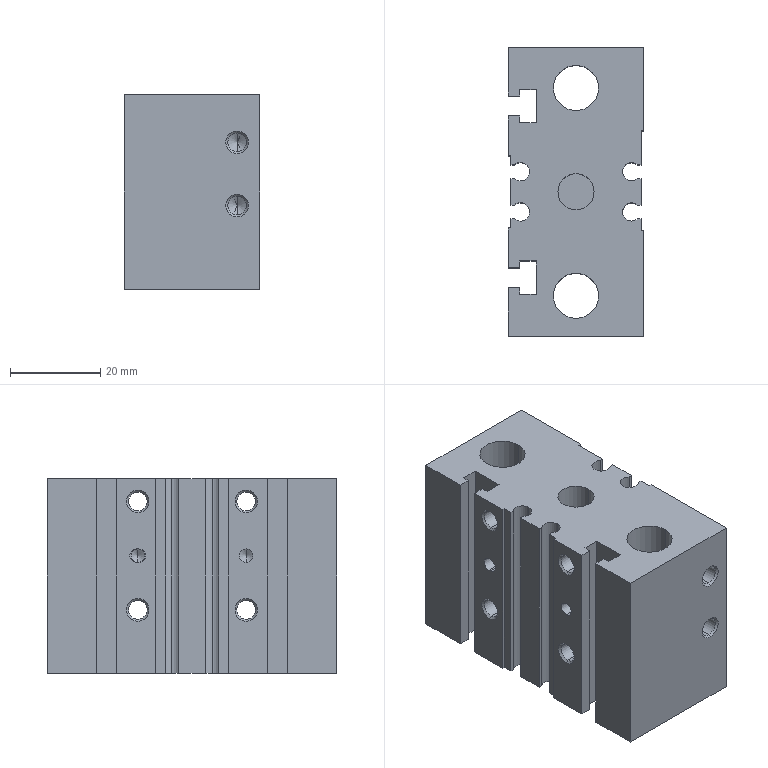Part | SolidWorks | features RefAxis 15, HoleWzd 11, 3DProfileFeature 5, RevCut 5, ICE 2, Extrusion 1, LPattern 1 | 1 solid | 178 faces | box 30 x 64 x 43 mm | volume 62167 mm3 | cylinder 66 | plane 64 | cone 48 | commonest cylinder face diameters 4.134 x24 3 x12 8 x10 4.3 x8 4.05 x6 10 x4